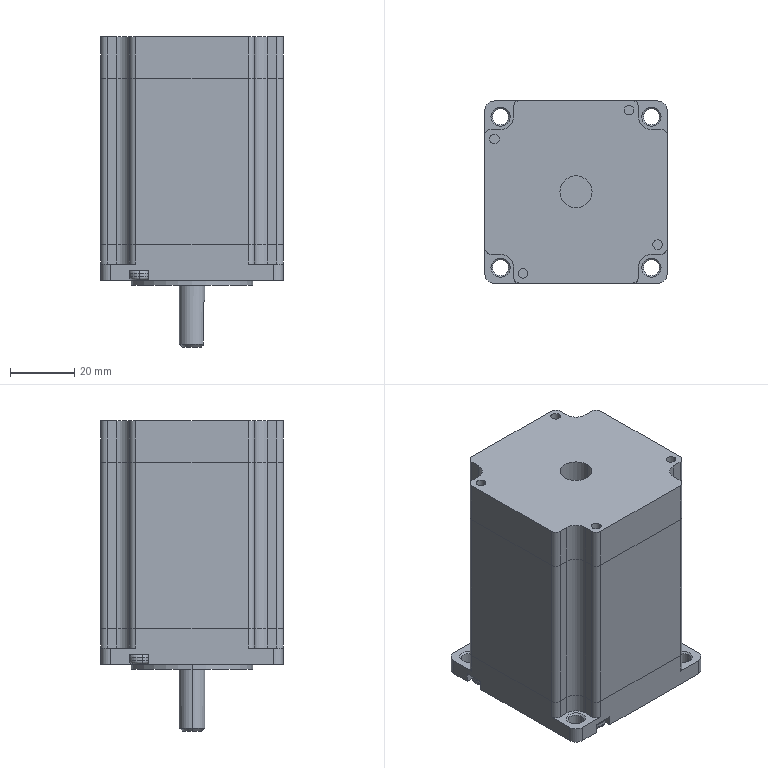Part | SolidWorks | 8 solids | 273 faces | box 57 x 57 x 97 mm | volume 225839 mm3 | plane 160 | cylinder 83 | torus 20 | cone 10 | commonest cylinder face diameters 4 x24 6 x19 8 x16 3 x8 5 x8 10 x6